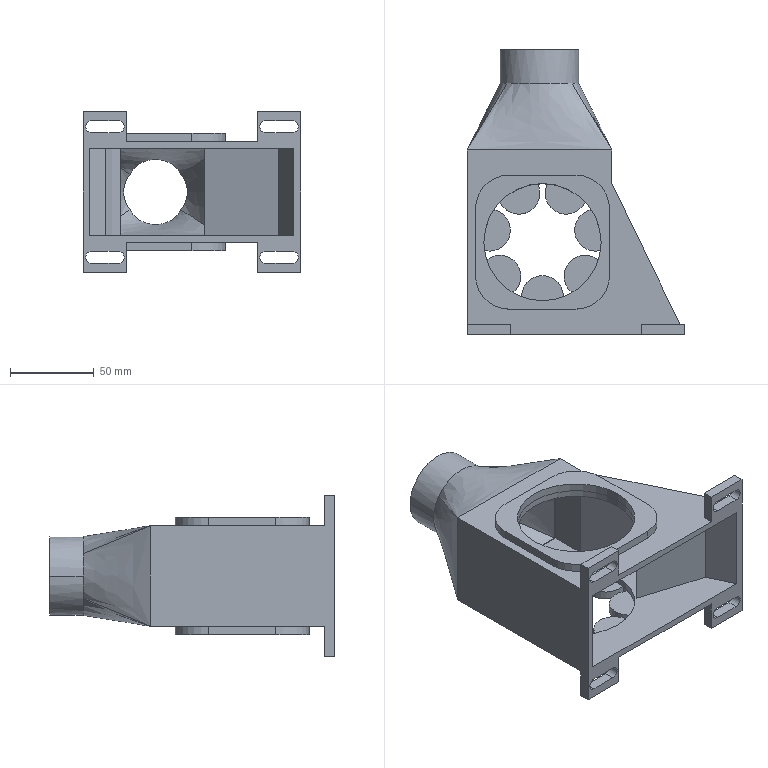Part | SolidWorks | features ICE 8, Blend 1, Extrusion 1, Shell 1 | 4 solids | 114 faces | box 130 x 170 x 96 mm | volume 239654 mm3 | plane 56 | cylinder 46 | spline 12 | commonest cylinder face diameters 70 x13 25.003 x12 7 x8 40 x8 47 x2 74 x2